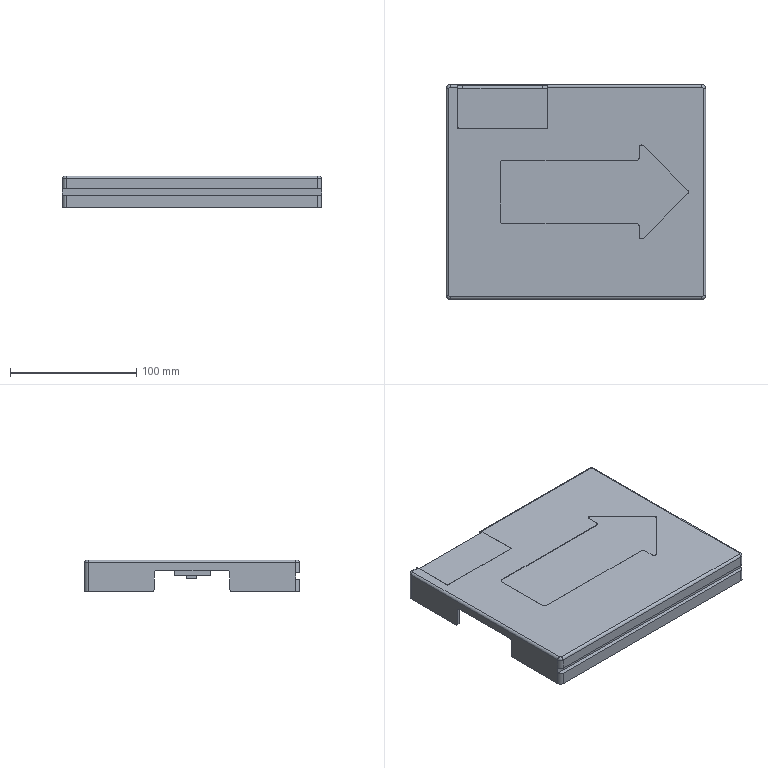Part | 3 solids | 180 faces | box 205 x 170 x 25 mm | volume 189620 mm3 | plane 98 | cylinder 66 | cone 12 | torus 4 | commonest cylinder face diameters 4 x31 6 x20 2.5 x15